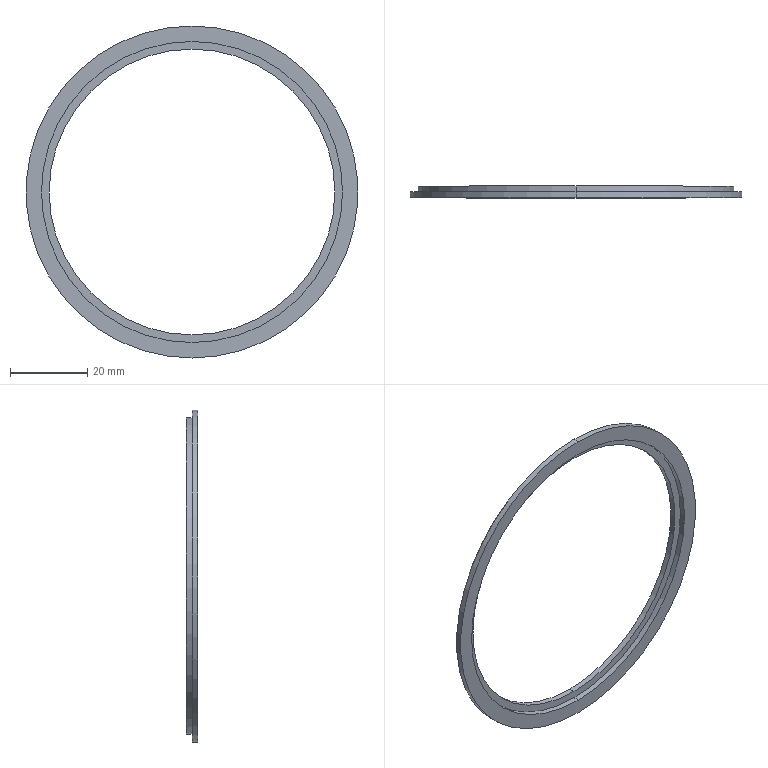Part | SolidWorks | features Revolution 1 | 1 solid | 12 faces | box 86 x 3 x 86 mm | volume 3016 mm3 | cylinder 8 | plane 4 | commonest cylinder face diameters 74 x2 78 x2 82 x2 86 x2
STEP:
#1=CARTESIAN_POINT('',(0.,-1.5,39.));
#2=VERTEX_POINT('',#1);
#3=CARTESIAN_POINT('',(0.,-1.5,-39.));
#4=VERTEX_POINT('',#3);
#5=CARTESIAN_POINT('',(0.,-1.5,0.));
#6=DIRECTION('',(0.,-1.,0.));
#7=DIRECTION('',(0.,0.,-1.));
#8=AXIS2_PLACEMENT_3D('',#5,#6,#7);
#9=CIRCLE('',#8,39.);
#10=EDGE_CURVE('',#2,#4,#9,.T.);
#11=ORIENTED_EDGE('',*,*,#10,.F.);
#12=CARTESIAN_POINT('',(0.,-3.,39.));
#13=VERTEX_POINT('',#12);
#14=CARTESIAN_POINT('',(0.,0.,39.));
#15=DIRECTION('',(0.,-1.,0.));
#16=VECTOR('',#15,1000.);
#17=LINE('',#14,#16);
#18=EDGE_CURVE('',#2,#13,#17,.T.);
#19=ORIENTED_EDGE('',*,*,#18,.T.);
#20=CARTESIAN_POINT('',(0.,-3.,-39.));
#21=VERTEX_POINT('',#20);
#22=CARTESIAN_POINT('',(0.,-3.,0.));
#23=DIRECTION('',(0.,-1.,0.));
#24=DIRECTION('',(0.,0.,-1.));
#25=AXIS2_PLACEMENT_3D('',#22,#23,#24);
#26=CIRCLE('',#25,39.);
#27=EDGE_CURVE('',#13,#21,#26,.T.);
#28=ORIENTED_EDGE('',*,*,#27,.T.);
#29=CARTESIAN_POINT('',(0.,0.,-39.));
#30=DIRECTION('',(0.,-1.,0.));
#31=VECTOR('',#30,1000.);
#32=LINE('',#29,#31);
#33=EDGE_CURVE('',#4,#21,#32,.T.);
#34=ORIENTED_EDGE('',*,*,#33,.F.);
#35=EDGE_LOOP('',(#11,#19,#28,#34));
#36=FACE_OUTER_BOUND('',#35,.T.);
#37=CARTESIAN_POINT('',(0.,0.,0.));
#38=DIRECTION('',(0.,-1.,0.));
#39=DIRECTION('',(0.,0.,-1.));
#40=AXIS2_PLACEMENT_3D('',#37,#38,#39);
#41=CYLINDRICAL_SURFACE('',#40,39.);
#42=ADVANCED_FACE('',(#36),#41,.F.);
#43=CARTESIAN_POINT('',(0.,-1.5,-43.));
#44=VERTEX_POINT('',#43);
#45=CARTESIAN_POINT('',(0.,-1.5,43.));
#46=VERTEX_POINT('',#45);
#47=CARTESIAN_POINT('',(0.,-1.5,0.));
#48=DIRECTION('',(0.,-1.,0.));
#49=DIRECTION('',(0.,0.,-1.));
#50=AXIS2_PLACEMENT_3D('',#47,#48,#49);
#51=CIRCLE('',#50,43.);
#52=EDGE_CURVE('',#44,#46,#51,.T.);
#53=ORIENTED_EDGE('',*,*,#52,.T.);
#54=CARTESIAN_POINT('',(0.,-3.,43.));
#55=VERTEX_POINT('',#54);
#56=CARTESIAN_POINT('',(0.,0.,43.));
#57=DIRECTION('',(0.,-1.,0.));
#58=VECTOR('',#57,1000.);
#59=LINE('',#56,#58);
#60=EDGE_CURVE('',#46,#55,#59,.T.);
#61=ORIENTED_EDGE('',*,*,#60,.T.);
#62=CARTESIAN_POINT('',(0.,-3.,-43.));
#63=VERTEX_POINT('',#62);
#64=CARTESIAN_POINT('',(0.,-3.,0.));
#65=DIRECTION('',(0.,-1.,0.));
#66=DIRECTION('',(0.,0.,-1.));
#67=AXIS2_PLACEMENT_3D('',#64,#65,#66);
#68=CIRCLE('',#67,43.);
#69=EDGE_CURVE('',#63,#55,#68,.T.);
#70=ORIENTED_EDGE('',*,*,#69,.F.);
#71=CARTESIAN_POINT('',(0.,0.,-43.));
#72=DIRECTION('',(0.,-1.,0.));
#73=VECTOR('',#72,1000.);
#74=LINE('',#71,#73);
#75=EDGE_CURVE('',#44,#63,#74,.T.);
#76=ORIENTED_EDGE('',*,*,#75,.F.);
#77=EDGE_LOOP('',(#53,#61,#70,#76));
#78=FACE_OUTER_BOUND('',#77,.T.);
#79=CARTESIAN_POINT('',(0.,0.,0.));
#80=DIRECTION('',(0.,-1.,0.));
#81=DIRECTION('',(0.,0.,-1.));
#82=AXIS2_PLACEMENT_3D('',#79,#80,#81);
#83=CYLINDRICAL_SURFACE('',#82,43.);
#84=ADVANCED_FACE('',(#78),#83,.T.);
#85=CARTESIAN_POINT('',(0.,0.,-41.));
#86=VERTEX_POINT('',#85);
#87=CARTESIAN_POINT('',(0.,0.,41.));
#88=VERTEX_POINT('',#87);
#89=CARTESIAN_POINT('',(0.,0.,0.));
#90=DIRECTION('',(0.,-1.,0.));
#91=DIRECTION('',(0.,0.,-1.));
#92=AXIS2_PLACEMENT_3D('',#89,#90,#91);
#93=CIRCLE('',#92,41.);
#94=EDGE_CURVE('',#86,#88,#93,.T.);
#95=ORIENTED_EDGE('',*,*,#94,.T.);
#96=CARTESIAN_POINT('',(0.,-1.5,41.));
#97=VERTEX_POINT('',#96);
#98=CARTESIAN_POINT('',(0.,0.,41.));
#99=DIRECTION('',(0.,-1.,0.));
#100=VECTOR('',#99,1000.);
#101=LINE('',#98,#100);
#102=EDGE_CURVE('',#88,#97,#101,.T.);
#103=ORIENTED_EDGE('',*,*,#102,.T.);
#104=CARTESIAN_POINT('',(0.,-1.5,-41.));
#105=VERTEX_POINT('',#104);
#106=CARTESIAN_POINT('',(0.,-1.5,0.));
#107=DIRECTION('',(0.,-1.,0.));
#108=DIRECTION('',(0.,0.,-1.));
#109=AXIS2_PLACEMENT_3D('',#106,#107,#108);
#110=CIRCLE('',#109,41.);
#111=EDGE_CURVE('',#105,#97,#110,.T.);
#112=ORIENTED_EDGE('',*,*,#111,.F.);
#113=CARTESIAN_POINT('',(0.,0.,-41.));
#114=DIRECTION('',(0.,-1.,0.));
#115=VECTOR('',#114,1000.);
#116=LINE('',#113,#115);
#117=EDGE_CURVE('',#86,#105,#116,.T.);
#118=ORIENTED_EDGE('',*,*,#117,.F.);
#119=EDGE_LOOP('',(#95,#103,#112,#118));
#120=FACE_OUTER_BOUND('',#119,.T.);
#121=CARTESIAN_POINT('',(0.,0.,0.));
#122=DIRECTION('',(0.,-1.,0.));
#123=DIRECTION('',(0.,0.,-1.));
#124=AXIS2_PLACEMENT_3D('',#121,#122,#123);
#125=CYLINDRICAL_SURFACE('',#124,41.);
#126=ADVANCED_FACE('',(#120),#125,.T.);
#127=CARTESIAN_POINT('',(0.,0.,37.));
#128=VERTEX_POINT('',#127);
#129=CARTESIAN_POINT('',(0.,0.,-37.));
#130=VERTEX_POINT('',#129);
#131=CARTESIAN_POINT('',(0.,0.,0.));
#132=DIRECTION('',(0.,-1.,0.));
#133=DIRECTION('',(0.,0.,-1.));
#134=AXIS2_PLACEMENT_3D('',#131,#132,#133);
#135=CIRCLE('',#134,37.);
#136=EDGE_CURVE('',#128,#130,#135,.T.);
#137=ORIENTED_EDGE('',*,*,#136,.F.);
#138=CARTESIAN_POINT('',(0.,-1.5,37.));
#139=VERTEX_POINT('',#138);
#140=CARTESIAN_POINT('',(0.,0.,37.));
#141=DIRECTION('',(0.,-1.,0.));
#142=VECTOR('',#141,1000.);
#143=LINE('',#140,#142);
#144=EDGE_CURVE('',#128,#139,#143,.T.);
#145=ORIENTED_EDGE('',*,*,#144,.T.);
#146=CARTESIAN_POINT('',(0.,-1.5,-37.));
#147=VERTEX_POINT('',#146);
#148=CARTESIAN_POINT('',(0.,-1.5,0.));
#149=DIRECTION('',(0.,-1.,0.));
#150=DIRECTION('',(0.,0.,-1.));
#151=AXIS2_PLACEMENT_3D('',#148,#149,#150);
#152=CIRCLE('',#151,37.);
#153=EDGE_CURVE('',#139,#147,#152,.T.);
#154=ORIENTED_EDGE('',*,*,#153,.T.);
#155=CARTESIAN_POINT('',(0.,0.,-37.));
#156=DIRECTION('',(0.,-1.,0.));
#157=VECTOR('',#156,1000.);
#158=LINE('',#155,#157);
#159=EDGE_CURVE('',#130,#147,#158,.T.);
#160=ORIENTED_EDGE('',*,*,#159,.F.);
#161=EDGE_LOOP('',(#137,#145,#154,#160));
#162=FACE_OUTER_BOUND('',#161,.T.);
#163=CARTESIAN_POINT('',(0.,0.,0.));
#164=DIRECTION('',(0.,-1.,0.));
#165=DIRECTION('',(0.,0.,-1.));
#166=AXIS2_PLACEMENT_3D('',#163,#164,#165);
#167=CYLINDRICAL_SURFACE('',#166,37.);
#168=ADVANCED_FACE('',(#162),#167,.F.);
#169=ORIENTED_EDGE('',*,*,#144,.F.);
#170=CARTESIAN_POINT('',(0.,0.,0.));
#171=DIRECTION('',(0.,-1.,0.));
#172=DIRECTION('',(0.,0.,-1.));
#173=AXIS2_PLACEMENT_3D('',#170,#171,#172);
#174=CIRCLE('',#173,37.);
#175=EDGE_CURVE('',#130,#128,#174,.T.);
#176=ORIENTED_EDGE('',*,*,#175,.F.);
#177=ORIENTED_EDGE('',*,*,#159,.T.);
#178=CARTESIAN_POINT('',(0.,-1.5,0.));
#179=DIRECTION('',(0.,-1.,0.));
#180=DIRECTION('',(0.,0.,-1.));
#181=AXIS2_PLACEMENT_3D('',#178,#179,#180);
#182=CIRCLE('',#181,37.);
#183=EDGE_CURVE('',#147,#139,#182,.T.);
#184=ORIENTED_EDGE('',*,*,#183,.T.);
#185=EDGE_LOOP('',(#169,#176,#177,#184));
#186=FACE_OUTER_BOUND('',#185,.T.);
#187=CARTESIAN_POINT('',(0.,0.,0.));
#188=DIRECTION('',(0.,-1.,0.));
#189=DIRECTION('',(0.,0.,-1.));
#190=AXIS2_PLACEMENT_3D('',#187,#188,#189);
#191=CYLINDRICAL_SURFACE('',#190,37.);
#192=ADVANCED_FACE('',(#186),#191,.F.);
#193=ORIENTED_EDGE('',*,*,#94,.F.);
#194=CARTESIAN_POINT('',(0.,0.,0.));
#195=DIRECTION('',(0.,-1.,0.));
#196=DIRECTION('',(0.,0.,-1.));
#197=AXIS2_PLACEMENT_3D('',#194,#195,#196);
#198=CIRCLE('',#197,41.);
#199=EDGE_CURVE('',#88,#86,#198,.T.);
#200=ORIENTED_EDGE('',*,*,#199,.F.);
#201=EDGE_LOOP('',(#193,#200));
#202=FACE_OUTER_BOUND('',#201,.T.);
#203=ORIENTED_EDGE('',*,*,#175,.T.);
#204=ORIENTED_EDGE('',*,*,#136,.T.);
#205=EDGE_LOOP('',(#203,#204));
#206=FACE_BOUND('',#205,.T.);
#207=CARTESIAN_POINT('',(-37.,0.,0.));
#208=DIRECTION('',(0.,-1.,0.));
#209=DIRECTION('',(0.,0.,-1.));
#210=AXIS2_PLACEMENT_3D('',#207,#208,#209);
#211=PLANE('',#210);
#212=ADVANCED_FACE('',(#202,#206),#211,.F.);
#213=ORIENTED_EDGE('',*,*,#102,.F.);
#214=ORIENTED_EDGE('',*,*,#199,.T.);
#215=ORIENTED_EDGE('',*,*,#117,.T.);
#216=CARTESIAN_POINT('',(0.,-1.5,0.));
#217=DIRECTION('',(0.,-1.,0.));
#218=DIRECTION('',(0.,0.,-1.));
#219=AXIS2_PLACEMENT_3D('',#216,#217,#218);
#220=CIRCLE('',#219,41.);
#221=EDGE_CURVE('',#97,#105,#220,.T.);
#222=ORIENTED_EDGE('',*,*,#221,.F.);
#223=EDGE_LOOP('',(#213,#214,#215,#222));
#224=FACE_OUTER_BOUND('',#223,.T.);
#225=CARTESIAN_POINT('',(0.,0.,0.));
#226=DIRECTION('',(0.,-1.,0.));
#227=DIRECTION('',(0.,0.,-1.));
#228=AXIS2_PLACEMENT_3D('',#225,#226,#227);
#229=CYLINDRICAL_SURFACE('',#228,41.);
#230=ADVANCED_FACE('',(#224),#229,.T.);
#231=ORIENTED_EDGE('',*,*,#52,.F.);
#232=CARTESIAN_POINT('',(0.,-1.5,0.));
#233=DIRECTION('',(0.,-1.,0.));
#234=DIRECTION('',(0.,0.,-1.));
#235=AXIS2_PLACEMENT_3D('',#232,#233,#234);
#236=CIRCLE('',#235,43.);
#237=EDGE_CURVE('',#46,#44,#236,.T.);
#238=ORIENTED_EDGE('',*,*,#237,.F.);
#239=EDGE_LOOP('',(#231,#238));
#240=FACE_OUTER_BOUND('',#239,.T.);
#241=ORIENTED_EDGE('',*,*,#111,.T.);
#242=ORIENTED_EDGE('',*,*,#221,.T.);
#243=EDGE_LOOP('',(#241,#242));
#244=FACE_BOUND('',#243,.T.);
#245=CARTESIAN_POINT('',(-41.,-1.5,0.));
#246=DIRECTION('',(0.,-1.,0.));
#247=DIRECTION('',(0.,0.,-1.));
#248=AXIS2_PLACEMENT_3D('',#245,#246,#247);
#249=PLANE('',#248);
#250=ADVANCED_FACE('',(#240,#244),#249,.F.);
#251=ORIENTED_EDGE('',*,*,#60,.F.);
#252=ORIENTED_EDGE('',*,*,#237,.T.);
#253=ORIENTED_EDGE('',*,*,#75,.T.);
#254=CARTESIAN_POINT('',(0.,-3.,0.));
#255=DIRECTION('',(0.,-1.,0.));
#256=DIRECTION('',(0.,0.,-1.));
#257=AXIS2_PLACEMENT_3D('',#254,#255,#256);
#258=CIRCLE('',#257,43.);
#259=EDGE_CURVE('',#55,#63,#258,.T.);
#260=ORIENTED_EDGE('',*,*,#259,.F.);
#261=EDGE_LOOP('',(#251,#252,#253,#260));
#262=FACE_OUTER_BOUND('',#261,.T.);
#263=CARTESIAN_POINT('',(0.,0.,0.));
#264=DIRECTION('',(0.,-1.,0.));
#265=DIRECTION('',(0.,0.,-1.));
#266=AXIS2_PLACEMENT_3D('',#263,#264,#265);
#267=CYLINDRICAL_SURFACE('',#266,43.);
#268=ADVANCED_FACE('',(#262),#267,.T.);
#269=CARTESIAN_POINT('',(0.,-3.,0.));
#270=DIRECTION('',(0.,-1.,0.));
#271=DIRECTION('',(0.,0.,-1.));
#272=AXIS2_PLACEMENT_3D('',#269,#270,#271);
#273=CIRCLE('',#272,39.);
#274=EDGE_CURVE('',#21,#13,#273,.T.);
#275=ORIENTED_EDGE('',*,*,#274,.F.);
#276=ORIENTED_EDGE('',*,*,#27,.F.);
#277=EDGE_LOOP('',(#275,#276));
#278=FACE_BOUND('',#277,.T.);
#279=ORIENTED_EDGE('',*,*,#69,.T.);
#280=ORIENTED_EDGE('',*,*,#259,.T.);
#281=EDGE_LOOP('',(#279,#280));
#282=FACE_OUTER_BOUND('',#281,.T.);
#283=CARTESIAN_POINT('',(-43.,-3.,0.));
#284=DIRECTION('',(0.,1.,0.));
#285=DIRECTION('',(0.,0.,1.));
#286=AXIS2_PLACEMENT_3D('',#283,#284,#285);
#287=PLANE('',#286);
#288=ADVANCED_FACE('',(#278,#282),#287,.F.);
#289=ORIENTED_EDGE('',*,*,#18,.F.);
#290=CARTESIAN_POINT('',(0.,-1.5,0.));
#291=DIRECTION('',(0.,-1.,0.));
#292=DIRECTION('',(0.,0.,-1.));
#293=AXIS2_PLACEMENT_3D('',#290,#291,#292);
#294=CIRCLE('',#293,39.);
#295=EDGE_CURVE('',#4,#2,#294,.T.);
#296=ORIENTED_EDGE('',*,*,#295,.F.);
#297=ORIENTED_EDGE('',*,*,#33,.T.);
#298=ORIENTED_EDGE('',*,*,#274,.T.);
#299=EDGE_LOOP('',(#289,#296,#297,#298));
#300=FACE_OUTER_BOUND('',#299,.T.);
#301=CARTESIAN_POINT('',(0.,0.,0.));
#302=DIRECTION('',(0.,-1.,0.));
#303=DIRECTION('',(0.,0.,-1.));
#304=AXIS2_PLACEMENT_3D('',#301,#302,#303);
#305=CYLINDRICAL_SURFACE('',#304,39.);
#306=ADVANCED_FACE('',(#300),#305,.F.);
#307=ORIENTED_EDGE('',*,*,#183,.F.);
#308=ORIENTED_EDGE('',*,*,#153,.F.);
#309=EDGE_LOOP('',(#307,#308));
#310=FACE_BOUND('',#309,.T.);
#311=ORIENTED_EDGE('',*,*,#295,.T.);
#312=ORIENTED_EDGE('',*,*,#10,.T.);
#313=EDGE_LOOP('',(#311,#312));
#314=FACE_OUTER_BOUND('',#313,.T.);
#315=CARTESIAN_POINT('',(-39.,-1.5,0.));
#316=DIRECTION('',(0.,1.,0.));
#317=DIRECTION('',(0.,0.,1.));
#318=AXIS2_PLACEMENT_3D('',#315,#316,#317);
#319=PLANE('',#318);
#320=ADVANCED_FACE('',(#310,#314),#319,.F.);
#321=CLOSED_SHELL('',(#42,#84,#126,#168,#192,#212,#230,#250,#268,#288,#306,#320));
#322=MANIFOLD_SOLID_BREP('',#321);
#323=CARTESIAN_POINT('',(0.,0.,0.));
#324=DIRECTION('',(0.,0.,1.));
#325=DIRECTION('',(1.,0.,0.));
#326=AXIS2_PLACEMENT_3D('',#323,#324,#325);
#327=(LENGTH_UNIT()NAMED_UNIT(*)SI_UNIT(.MILLI.,.METRE.));
#328=UNCERTAINTY_MEASURE_WITH_UNIT(LENGTH_MEASURE(0.00001),#327,'','');
#329=(NAMED_UNIT(*)PLANE_ANGLE_UNIT()SI_UNIT($,.RADIAN.));
#330=(NAMED_UNIT(*)SI_UNIT($,.STERADIAN.)SOLID_ANGLE_UNIT());
#331=(GEOMETRIC_REPRESENTATION_CONTEXT(3)GLOBAL_UNCERTAINTY_ASSIGNED_CONTEXT((#328))GLOBAL_UNIT_ASSIGNED_CONTEXT((#327,#329,#330))REPRESENTATION_CONTEXT('',''));
#332=ADVANCED_BREP_SHAPE_REPRESENTATION('',(#322,#326),#331);